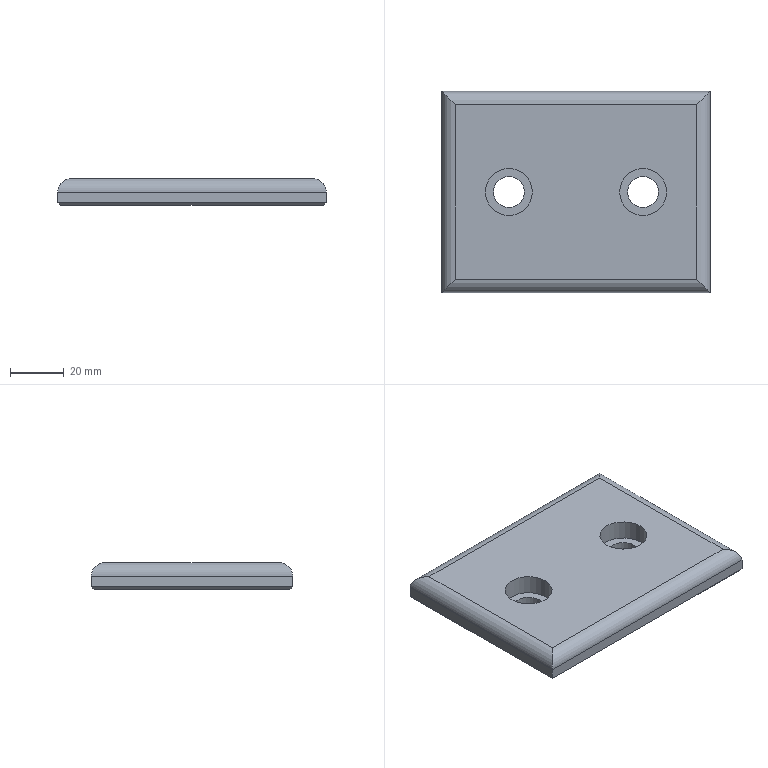Part | NX | features solid 2 | 1 solid | 20 faces | box 100 x 75 x 10 mm | volume 68924 mm3 | plane 12 | cylinder 8 | commonest cylinder face diameters 10 x4 11.5 x2 17.5 x2
STEP:
#1=CARTESIAN_POINT('',(660.,-700.,-129.));
#2=VERTEX_POINT('',#1);
#3=CARTESIAN_POINT('',(660.,-700.,-125.));
#4=VERTEX_POINT('',#3);
#5=CARTESIAN_POINT('',(660.,-700.,-130.));
#6=DIRECTION('',(0.,0.,1.));
#7=VECTOR('',#6,1000.);
#8=LINE('',#5,#7);
#9=EDGE_CURVE('',#2,#4,#8,.T.);
#10=ORIENTED_EDGE('',*,*,#9,.T.);
#11=CARTESIAN_POINT('',(660.,-625.,-125.));
#12=VERTEX_POINT('',#11);
#13=CARTESIAN_POINT('',(660.,-700.,-125.));
#14=DIRECTION('',(0.,-1.,0.));
#15=VECTOR('',#14,1000.);
#16=LINE('',#13,#15);
#17=EDGE_CURVE('',#12,#4,#16,.T.);
#18=ORIENTED_EDGE('',*,*,#17,.F.);
#19=CARTESIAN_POINT('',(660.,-625.,-129.));
#20=VERTEX_POINT('',#19);
#21=CARTESIAN_POINT('',(660.,-625.,-130.));
#22=DIRECTION('',(0.,0.,1.));
#23=VECTOR('',#22,1000.);
#24=LINE('',#21,#23);
#25=EDGE_CURVE('',#20,#12,#24,.T.);
#26=ORIENTED_EDGE('',*,*,#25,.F.);
#27=CARTESIAN_POINT('',(660.,-625.,-129.));
#28=DIRECTION('',(0.,1.,0.));
#29=VECTOR('',#28,1000.);
#30=LINE('',#27,#29);
#31=EDGE_CURVE('',#2,#20,#30,.T.);
#32=ORIENTED_EDGE('',*,*,#31,.F.);
#33=EDGE_LOOP('',(#10,#18,#26,#32));
#34=FACE_BOUND('',#33,.T.);
#35=CARTESIAN_POINT('',(660.,-625.,-130.));
#36=DIRECTION('',(1.,0.,0.));
#37=DIRECTION('',(0.,-1.,0.));
#38=AXIS2_PLACEMENT_3D('',#35,#36,#37);
#39=PLANE('',#38);
#40=ADVANCED_FACE('',(#34),#39,.F.);
#41=CARTESIAN_POINT('',(760.,-700.,-129.));
#42=VERTEX_POINT('',#41);
#43=CARTESIAN_POINT('',(760.,-700.,-125.));
#44=VERTEX_POINT('',#43);
#45=CARTESIAN_POINT('',(760.,-700.,-130.));
#46=DIRECTION('',(0.,0.,1.));
#47=VECTOR('',#46,1000.);
#48=LINE('',#45,#47);
#49=EDGE_CURVE('',#42,#44,#48,.T.);
#50=ORIENTED_EDGE('',*,*,#49,.T.);
#51=CARTESIAN_POINT('',(760.,-700.,-125.));
#52=DIRECTION('',(1.,0.,0.));
#53=VECTOR('',#52,1000.);
#54=LINE('',#51,#53);
#55=EDGE_CURVE('',#4,#44,#54,.T.);
#56=ORIENTED_EDGE('',*,*,#55,.F.);
#57=ORIENTED_EDGE('',*,*,#9,.F.);
#58=CARTESIAN_POINT('',(660.,-700.,-129.));
#59=DIRECTION('',(-1.,0.,0.));
#60=VECTOR('',#59,1000.);
#61=LINE('',#58,#60);
#62=EDGE_CURVE('',#42,#2,#61,.T.);
#63=ORIENTED_EDGE('',*,*,#62,.F.);
#64=EDGE_LOOP('',(#50,#56,#57,#63));
#65=FACE_BOUND('',#64,.T.);
#66=CARTESIAN_POINT('',(660.,-700.,-130.));
#67=DIRECTION('',(0.,1.,0.));
#68=DIRECTION('',(1.,0.,0.));
#69=AXIS2_PLACEMENT_3D('',#66,#67,#68);
#70=PLANE('',#69);
#71=ADVANCED_FACE('',(#65),#70,.F.);
#72=CARTESIAN_POINT('',(760.,-625.,-129.));
#73=VERTEX_POINT('',#72);
#74=CARTESIAN_POINT('',(760.,-625.,-125.));
#75=VERTEX_POINT('',#74);
#76=CARTESIAN_POINT('',(760.,-625.,-130.));
#77=DIRECTION('',(0.,0.,1.));
#78=VECTOR('',#77,1000.);
#79=LINE('',#76,#78);
#80=EDGE_CURVE('',#73,#75,#79,.T.);
#81=ORIENTED_EDGE('',*,*,#80,.T.);
#82=CARTESIAN_POINT('',(760.,-625.,-125.));
#83=DIRECTION('',(0.,1.,0.));
#84=VECTOR('',#83,1000.);
#85=LINE('',#82,#84);
#86=EDGE_CURVE('',#44,#75,#85,.T.);
#87=ORIENTED_EDGE('',*,*,#86,.F.);
#88=ORIENTED_EDGE('',*,*,#49,.F.);
#89=CARTESIAN_POINT('',(760.,-700.,-129.));
#90=DIRECTION('',(0.,-1.,0.));
#91=VECTOR('',#90,1000.);
#92=LINE('',#89,#91);
#93=EDGE_CURVE('',#73,#42,#92,.T.);
#94=ORIENTED_EDGE('',*,*,#93,.F.);
#95=EDGE_LOOP('',(#81,#87,#88,#94));
#96=FACE_BOUND('',#95,.T.);
#97=CARTESIAN_POINT('',(760.,-700.,-130.));
#98=DIRECTION('',(-1.,0.,0.));
#99=DIRECTION('',(0.,1.,0.));
#100=AXIS2_PLACEMENT_3D('',#97,#98,#99);
#101=PLANE('',#100);
#102=ADVANCED_FACE('',(#96),#101,.F.);
#103=ORIENTED_EDGE('',*,*,#25,.T.);
#104=CARTESIAN_POINT('',(660.,-625.,-125.));
#105=DIRECTION('',(-1.,0.,0.));
#106=VECTOR('',#105,1000.);
#107=LINE('',#104,#106);
#108=EDGE_CURVE('',#75,#12,#107,.T.);
#109=ORIENTED_EDGE('',*,*,#108,.F.);
#110=ORIENTED_EDGE('',*,*,#80,.F.);
#111=CARTESIAN_POINT('',(760.,-625.,-129.));
#112=DIRECTION('',(1.,0.,0.));
#113=VECTOR('',#112,1000.);
#114=LINE('',#111,#113);
#115=EDGE_CURVE('',#20,#73,#114,.T.);
#116=ORIENTED_EDGE('',*,*,#115,.F.);
#117=EDGE_LOOP('',(#103,#109,#110,#116));
#118=FACE_BOUND('',#117,.T.);
#119=CARTESIAN_POINT('',(760.,-625.,-130.));
#120=DIRECTION('',(0.,-1.,0.));
#121=DIRECTION('',(-1.,0.,0.));
#122=AXIS2_PLACEMENT_3D('',#119,#120,#121);
#123=PLANE('',#122);
#124=ADVANCED_FACE('',(#118),#123,.F.);
#125=CARTESIAN_POINT('',(661.,-626.,-130.));
#126=VERTEX_POINT('',#125);
#127=CARTESIAN_POINT('',(661.,-699.,-130.));
#128=VERTEX_POINT('',#127);
#129=CARTESIAN_POINT('',(661.,-625.,-130.));
#130=DIRECTION('',(0.,-1.,0.));
#131=VECTOR('',#130,1000.);
#132=LINE('',#129,#131);
#133=EDGE_CURVE('',#126,#128,#132,.T.);
#134=ORIENTED_EDGE('',*,*,#133,.F.);
#135=CARTESIAN_POINT('',(759.,-626.,-130.));
#136=VERTEX_POINT('',#135);
#137=CARTESIAN_POINT('',(660.,-626.,-130.));
#138=DIRECTION('',(-1.,0.,0.));
#139=VECTOR('',#138,1000.);
#140=LINE('',#137,#139);
#141=EDGE_CURVE('',#136,#126,#140,.T.);
#142=ORIENTED_EDGE('',*,*,#141,.F.);
#143=CARTESIAN_POINT('',(759.,-699.,-130.));
#144=VERTEX_POINT('',#143);
#145=CARTESIAN_POINT('',(759.,-625.,-130.));
#146=DIRECTION('',(0.,1.,0.));
#147=VECTOR('',#146,1000.);
#148=LINE('',#145,#147);
#149=EDGE_CURVE('',#144,#136,#148,.T.);
#150=ORIENTED_EDGE('',*,*,#149,.F.);
#151=CARTESIAN_POINT('',(660.,-699.,-130.));
#152=DIRECTION('',(1.,0.,0.));
#153=VECTOR('',#152,1000.);
#154=LINE('',#151,#153);
#155=EDGE_CURVE('',#128,#144,#154,.T.);
#156=ORIENTED_EDGE('',*,*,#155,.F.);
#157=EDGE_LOOP('',(#134,#142,#150,#156));
#158=FACE_BOUND('',#157,.T.);
#159=CARTESIAN_POINT('',(740.75,-662.5,-130.));
#160=VERTEX_POINT('',#159);
#161=CARTESIAN_POINT('',(735.,-662.5,-130.));
#162=DIRECTION('',(0.,0.,-1.));
#163=DIRECTION('',(1.,0.,0.));
#164=AXIS2_PLACEMENT_3D('',#161,#162,#163);
#165=CIRCLE('',#164,5.75);
#166=EDGE_CURVE('',#160,#160,#165,.T.);
#167=ORIENTED_EDGE('',*,*,#166,.F.);
#168=EDGE_LOOP('',(#167));
#169=FACE_BOUND('',#168,.T.);
#170=CARTESIAN_POINT('',(690.75,-662.5,-130.));
#171=VERTEX_POINT('',#170);
#172=CARTESIAN_POINT('',(685.,-662.5,-130.));
#173=DIRECTION('',(0.,0.,-1.));
#174=DIRECTION('',(1.,0.,0.));
#175=AXIS2_PLACEMENT_3D('',#172,#173,#174);
#176=CIRCLE('',#175,5.75);
#177=EDGE_CURVE('',#171,#171,#176,.T.);
#178=ORIENTED_EDGE('',*,*,#177,.F.);
#179=EDGE_LOOP('',(#178));
#180=FACE_BOUND('',#179,.T.);
#181=CARTESIAN_POINT('',(660.,-625.,-130.));
#182=DIRECTION('',(0.,0.,1.));
#183=DIRECTION('',(1.,0.,0.));
#184=AXIS2_PLACEMENT_3D('',#181,#182,#183);
#185=PLANE('',#184);
#186=ADVANCED_FACE('',(#158,#169,#180),#185,.F.);
#187=CARTESIAN_POINT('',(755.,-630.,-120.));
#188=VERTEX_POINT('',#187);
#189=CARTESIAN_POINT('',(755.,-695.,-120.));
#190=VERTEX_POINT('',#189);
#191=CARTESIAN_POINT('',(755.,-700.,-120.));
#192=DIRECTION('',(0.,1.,0.));
#193=VECTOR('',#192,1000.);
#194=LINE('',#191,#193);
#195=EDGE_CURVE('',#188,#190,#194,.F.);
#196=ORIENTED_EDGE('',*,*,#195,.F.);
#197=CARTESIAN_POINT('',(665.,-630.,-120.));
#198=VERTEX_POINT('',#197);
#199=CARTESIAN_POINT('',(760.,-630.,-120.));
#200=DIRECTION('',(-1.,0.,0.));
#201=VECTOR('',#200,1000.);
#202=LINE('',#199,#201);
#203=EDGE_CURVE('',#198,#188,#202,.F.);
#204=ORIENTED_EDGE('',*,*,#203,.F.);
#205=CARTESIAN_POINT('',(665.,-695.,-120.));
#206=VERTEX_POINT('',#205);
#207=CARTESIAN_POINT('',(665.,-625.,-120.));
#208=DIRECTION('',(0.,-1.,0.));
#209=VECTOR('',#208,1000.);
#210=LINE('',#207,#209);
#211=EDGE_CURVE('',#206,#198,#210,.F.);
#212=ORIENTED_EDGE('',*,*,#211,.F.);
#213=CARTESIAN_POINT('',(660.,-695.,-120.));
#214=DIRECTION('',(1.,0.,0.));
#215=VECTOR('',#214,1000.);
#216=LINE('',#213,#215);
#217=EDGE_CURVE('',#190,#206,#216,.F.);
#218=ORIENTED_EDGE('',*,*,#217,.F.);
#219=EDGE_LOOP('',(#196,#204,#212,#218));
#220=FACE_BOUND('',#219,.T.);
#221=CARTESIAN_POINT('',(726.25,-662.5,-120.));
#222=VERTEX_POINT('',#221);
#223=CARTESIAN_POINT('',(735.,-662.5,-120.));
#224=DIRECTION('',(0.,0.,1.));
#225=DIRECTION('',(-1.,0.,0.));
#226=AXIS2_PLACEMENT_3D('',#223,#224,#225);
#227=CIRCLE('',#226,8.75);
#228=EDGE_CURVE('',#222,#222,#227,.T.);
#229=ORIENTED_EDGE('',*,*,#228,.F.);
#230=EDGE_LOOP('',(#229));
#231=FACE_BOUND('',#230,.T.);
#232=CARTESIAN_POINT('',(676.25,-662.5,-120.));
#233=VERTEX_POINT('',#232);
#234=CARTESIAN_POINT('',(685.,-662.5,-120.));
#235=DIRECTION('',(0.,0.,1.));
#236=DIRECTION('',(-1.,0.,0.));
#237=AXIS2_PLACEMENT_3D('',#234,#235,#236);
#238=CIRCLE('',#237,8.75);
#239=EDGE_CURVE('',#233,#233,#238,.T.);
#240=ORIENTED_EDGE('',*,*,#239,.F.);
#241=EDGE_LOOP('',(#240));
#242=FACE_BOUND('',#241,.T.);
#243=CARTESIAN_POINT('',(660.,-625.,-120.));
#244=DIRECTION('',(0.,0.,1.));
#245=DIRECTION('',(1.,0.,0.));
#246=AXIS2_PLACEMENT_3D('',#243,#244,#245);
#247=PLANE('',#246);
#248=ADVANCED_FACE('',(#220,#231,#242),#247,.T.);
#249=CARTESIAN_POINT('',(679.25,-662.5,-127.3));
#250=VERTEX_POINT('',#249);
#251=CARTESIAN_POINT('',(685.,-662.5,-127.3));
#252=DIRECTION('',(0.,0.,1.));
#253=DIRECTION('',(-1.,0.,0.));
#254=AXIS2_PLACEMENT_3D('',#251,#252,#253);
#255=CIRCLE('',#254,5.75);
#256=EDGE_CURVE('',#250,#250,#255,.T.);
#257=ORIENTED_EDGE('',*,*,#256,.T.);
#258=EDGE_LOOP('',(#257));
#259=FACE_BOUND('',#258,.T.);
#260=ORIENTED_EDGE('',*,*,#177,.T.);
#261=EDGE_LOOP('',(#260));
#262=FACE_BOUND('',#261,.T.);
#263=CARTESIAN_POINT('',(685.,-662.5,-170.));
#264=DIRECTION('',(0.,0.,-1.));
#265=DIRECTION('',(-1.,0.,0.));
#266=AXIS2_PLACEMENT_3D('',#263,#264,#265);
#267=CYLINDRICAL_SURFACE('',#266,5.75);
#268=ADVANCED_FACE('',(#259,#262),#267,.F.);
#269=ORIENTED_EDGE('',*,*,#256,.F.);
#270=EDGE_LOOP('',(#269));
#271=FACE_BOUND('',#270,.T.);
#272=CARTESIAN_POINT('',(676.25,-662.5,-127.3));
#273=VERTEX_POINT('',#272);
#274=CARTESIAN_POINT('',(685.,-662.5,-127.3));
#275=DIRECTION('',(0.,0.,1.));
#276=DIRECTION('',(-1.,0.,0.));
#277=AXIS2_PLACEMENT_3D('',#274,#275,#276);
#278=CIRCLE('',#277,8.75);
#279=EDGE_CURVE('',#273,#273,#278,.T.);
#280=ORIENTED_EDGE('',*,*,#279,.T.);
#281=EDGE_LOOP('',(#280));
#282=FACE_BOUND('',#281,.T.);
#283=CARTESIAN_POINT('',(685.,-662.5,-127.3));
#284=DIRECTION('',(0.,0.,-1.));
#285=DIRECTION('',(-1.,0.,0.));
#286=AXIS2_PLACEMENT_3D('',#283,#284,#285);
#287=PLANE('',#286);
#288=ADVANCED_FACE('',(#271,#282),#287,.F.);
#289=ORIENTED_EDGE('',*,*,#279,.F.);
#290=EDGE_LOOP('',(#289));
#291=FACE_BOUND('',#290,.T.);
#292=ORIENTED_EDGE('',*,*,#239,.T.);
#293=EDGE_LOOP('',(#292));
#294=FACE_BOUND('',#293,.T.);
#295=CARTESIAN_POINT('',(685.,-662.5,-120.));
#296=DIRECTION('',(0.,0.,-1.));
#297=DIRECTION('',(-1.,0.,0.));
#298=AXIS2_PLACEMENT_3D('',#295,#296,#297);
#299=CYLINDRICAL_SURFACE('',#298,8.75);
#300=ADVANCED_FACE('',(#291,#294),#299,.F.);
#301=CARTESIAN_POINT('',(729.25,-662.5,-127.3));
#302=VERTEX_POINT('',#301);
#303=CARTESIAN_POINT('',(735.,-662.5,-127.3));
#304=DIRECTION('',(0.,0.,1.));
#305=DIRECTION('',(-1.,0.,0.));
#306=AXIS2_PLACEMENT_3D('',#303,#304,#305);
#307=CIRCLE('',#306,5.75);
#308=EDGE_CURVE('',#302,#302,#307,.T.);
#309=ORIENTED_EDGE('',*,*,#308,.T.);
#310=EDGE_LOOP('',(#309));
#311=FACE_BOUND('',#310,.T.);
#312=ORIENTED_EDGE('',*,*,#166,.T.);
#313=EDGE_LOOP('',(#312));
#314=FACE_BOUND('',#313,.T.);
#315=CARTESIAN_POINT('',(735.,-662.5,-170.));
#316=DIRECTION('',(0.,0.,-1.));
#317=DIRECTION('',(-1.,0.,0.));
#318=AXIS2_PLACEMENT_3D('',#315,#316,#317);
#319=CYLINDRICAL_SURFACE('',#318,5.75);
#320=ADVANCED_FACE('',(#311,#314),#319,.F.);
#321=ORIENTED_EDGE('',*,*,#308,.F.);
#322=EDGE_LOOP('',(#321));
#323=FACE_BOUND('',#322,.T.);
#324=CARTESIAN_POINT('',(726.25,-662.5,-127.3));
#325=VERTEX_POINT('',#324);
#326=CARTESIAN_POINT('',(735.,-662.5,-127.3));
#327=DIRECTION('',(0.,0.,1.));
#328=DIRECTION('',(-1.,0.,0.));
#329=AXIS2_PLACEMENT_3D('',#326,#327,#328);
#330=CIRCLE('',#329,8.75);
#331=EDGE_CURVE('',#325,#325,#330,.T.);
#332=ORIENTED_EDGE('',*,*,#331,.T.);
#333=EDGE_LOOP('',(#332));
#334=FACE_BOUND('',#333,.T.);
#335=CARTESIAN_POINT('',(735.,-662.5,-127.3));
#336=DIRECTION('',(0.,0.,-1.));
#337=DIRECTION('',(-1.,0.,0.));
#338=AXIS2_PLACEMENT_3D('',#335,#336,#337);
#339=PLANE('',#338);
#340=ADVANCED_FACE('',(#323,#334),#339,.F.);
#341=ORIENTED_EDGE('',*,*,#331,.F.);
#342=EDGE_LOOP('',(#341));
#343=FACE_BOUND('',#342,.T.);
#344=ORIENTED_EDGE('',*,*,#228,.T.);
#345=EDGE_LOOP('',(#344));
#346=FACE_BOUND('',#345,.T.);
#347=CARTESIAN_POINT('',(735.,-662.5,-120.));
#348=DIRECTION('',(0.,0.,-1.));
#349=DIRECTION('',(-1.,0.,0.));
#350=AXIS2_PLACEMENT_3D('',#347,#348,#349);
#351=CYLINDRICAL_SURFACE('',#350,8.75);
#352=ADVANCED_FACE('',(#343,#346),#351,.F.);
#353=CARTESIAN_POINT('',(755.,-630.,-125.));
#354=DIRECTION('',(-0.7071,0.7071,0.));
#355=DIRECTION('',(0.7071,0.7071,0.));
#356=AXIS2_PLACEMENT_3D('',#353,#354,#355);
#357=ELLIPSE('',#356,7.071,5.);
#358=EDGE_CURVE('',#188,#75,#357,.T.);
#359=ORIENTED_EDGE('',*,*,#358,.T.);
#360=ORIENTED_EDGE('',*,*,#108,.T.);
#361=CARTESIAN_POINT('',(665.,-630.,-125.));
#362=DIRECTION('',(-0.7071,-0.7071,0.));
#363=DIRECTION('',(-0.7071,0.7071,0.));
#364=AXIS2_PLACEMENT_3D('',#361,#362,#363);
#365=ELLIPSE('',#364,7.071,5.);
#366=EDGE_CURVE('',#12,#198,#365,.F.);
#367=ORIENTED_EDGE('',*,*,#366,.T.);
#368=ORIENTED_EDGE('',*,*,#203,.T.);
#369=EDGE_LOOP('',(#359,#360,#367,#368));
#370=FACE_BOUND('',#369,.T.);
#371=CARTESIAN_POINT('',(760.,-630.,-125.));
#372=DIRECTION('',(1.,0.,0.));
#373=DIRECTION('',(0.,-1.,0.));
#374=AXIS2_PLACEMENT_3D('',#371,#372,#373);
#375=CYLINDRICAL_SURFACE('',#374,5.);
#376=ADVANCED_FACE('',(#370),#375,.T.);
#377=ORIENTED_EDGE('',*,*,#366,.F.);
#378=ORIENTED_EDGE('',*,*,#17,.T.);
#379=CARTESIAN_POINT('',(665.,-695.,-125.));
#380=DIRECTION('',(0.7071,-0.7071,0.));
#381=DIRECTION('',(0.7071,0.7071,0.));
#382=AXIS2_PLACEMENT_3D('',#379,#380,#381);
#383=ELLIPSE('',#382,7.071,5.);
#384=EDGE_CURVE('',#4,#206,#383,.F.);
#385=ORIENTED_EDGE('',*,*,#384,.T.);
#386=ORIENTED_EDGE('',*,*,#211,.T.);
#387=EDGE_LOOP('',(#377,#378,#385,#386));
#388=FACE_BOUND('',#387,.T.);
#389=CARTESIAN_POINT('',(665.,-625.,-125.));
#390=DIRECTION('',(0.,1.,0.));
#391=DIRECTION('',(1.,0.,0.));
#392=AXIS2_PLACEMENT_3D('',#389,#390,#391);
#393=CYLINDRICAL_SURFACE('',#392,5.);
#394=ADVANCED_FACE('',(#388),#393,.T.);
#395=ORIENTED_EDGE('',*,*,#358,.F.);
#396=ORIENTED_EDGE('',*,*,#195,.T.);
#397=CARTESIAN_POINT('',(755.,-695.,-125.));
#398=DIRECTION('',(0.7071,0.7071,0.));
#399=DIRECTION('',(0.7071,-0.7071,0.));
#400=AXIS2_PLACEMENT_3D('',#397,#398,#399);
#401=ELLIPSE('',#400,7.071,5.);
#402=EDGE_CURVE('',#190,#44,#401,.T.);
#403=ORIENTED_EDGE('',*,*,#402,.T.);
#404=ORIENTED_EDGE('',*,*,#86,.T.);
#405=EDGE_LOOP('',(#395,#396,#403,#404));
#406=FACE_BOUND('',#405,.T.);
#407=CARTESIAN_POINT('',(755.,-700.,-125.));
#408=DIRECTION('',(0.,-1.,0.));
#409=DIRECTION('',(-1.,0.,0.));
#410=AXIS2_PLACEMENT_3D('',#407,#408,#409);
#411=CYLINDRICAL_SURFACE('',#410,5.);
#412=ADVANCED_FACE('',(#406),#411,.T.);
#413=ORIENTED_EDGE('',*,*,#384,.F.);
#414=ORIENTED_EDGE('',*,*,#55,.T.);
#415=ORIENTED_EDGE('',*,*,#402,.F.);
#416=ORIENTED_EDGE('',*,*,#217,.T.);
#417=EDGE_LOOP('',(#413,#414,#415,#416));
#418=FACE_BOUND('',#417,.T.);
#419=CARTESIAN_POINT('',(660.,-695.,-125.));
#420=DIRECTION('',(-1.,0.,0.));
#421=DIRECTION('',(0.,1.,0.));
#422=AXIS2_PLACEMENT_3D('',#419,#420,#421);
#423=CYLINDRICAL_SURFACE('',#422,5.);
#424=ADVANCED_FACE('',(#418),#423,.T.);
#425=CARTESIAN_POINT('',(726.,-659.,-163.));
#426=DIRECTION('',(0.5774,0.5774,0.5774));
#427=VECTOR('',#426,1000.);
#428=LINE('',#425,#427);
#429=EDGE_CURVE('',#73,#136,#428,.F.);
#430=ORIENTED_EDGE('',*,*,#429,.T.);
#431=ORIENTED_EDGE('',*,*,#141,.T.);
#432=CARTESIAN_POINT('',(660.667,-625.667,-129.667));
#433=DIRECTION('',(-0.5774,0.5774,0.5774));
#434=VECTOR('',#433,1000.);
#435=LINE('',#432,#434);
#436=EDGE_CURVE('',#126,#20,#435,.T.);
#437=ORIENTED_EDGE('',*,*,#436,.T.);
#438=ORIENTED_EDGE('',*,*,#115,.T.);
#439=EDGE_LOOP('',(#430,#431,#437,#438));
#440=FACE_BOUND('',#439,.T.);
#441=CARTESIAN_POINT('',(660.,-626.,-130.));
#442=DIRECTION('',(0.,-0.7071,0.7071));
#443=DIRECTION('',(0.,0.7071,0.7071));
#444=AXIS2_PLACEMENT_3D('',#441,#442,#443);
#445=PLANE('',#444);
#446=ADVANCED_FACE('',(#440),#445,.F.);
#447=ORIENTED_EDGE('',*,*,#436,.F.);
#448=ORIENTED_EDGE('',*,*,#133,.T.);
#449=CARTESIAN_POINT('',(685.667,-674.333,-154.667));
#450=DIRECTION('',(0.5774,0.5774,-0.5774));
#451=VECTOR('',#450,1000.);
#452=LINE('',#449,#451);
#453=EDGE_CURVE('',#128,#2,#452,.F.);
#454=ORIENTED_EDGE('',*,*,#453,.T.);
#455=ORIENTED_EDGE('',*,*,#31,.T.);
#456=EDGE_LOOP('',(#447,#448,#454,#455));
#457=FACE_BOUND('',#456,.T.);
#458=CARTESIAN_POINT('',(661.,-625.,-130.));
#459=DIRECTION('',(0.7071,0.,0.7071));
#460=DIRECTION('',(0.7071,0.,-0.7071));
#461=AXIS2_PLACEMENT_3D('',#458,#459,#460);
#462=PLANE('',#461);
#463=ADVANCED_FACE('',(#457),#462,.F.);
#464=ORIENTED_EDGE('',*,*,#429,.F.);
#465=ORIENTED_EDGE('',*,*,#93,.T.);
#466=CARTESIAN_POINT('',(734.333,-674.333,-154.667));
#467=DIRECTION('',(0.5774,-0.5774,0.5774));
#468=VECTOR('',#467,1000.);
#469=LINE('',#466,#468);
#470=EDGE_CURVE('',#42,#144,#469,.F.);
#471=ORIENTED_EDGE('',*,*,#470,.T.);
#472=ORIENTED_EDGE('',*,*,#149,.T.);
#473=EDGE_LOOP('',(#464,#465,#471,#472));
#474=FACE_BOUND('',#473,.T.);
#475=CARTESIAN_POINT('',(759.,-625.,-130.));
#476=DIRECTION('',(-0.7071,0.,0.7071));
#477=DIRECTION('',(0.7071,0.,0.7071));
#478=AXIS2_PLACEMENT_3D('',#475,#476,#477);
#479=PLANE('',#478);
#480=ADVANCED_FACE('',(#474),#479,.F.);
#481=ORIENTED_EDGE('',*,*,#453,.F.);
#482=ORIENTED_EDGE('',*,*,#155,.T.);
#483=ORIENTED_EDGE('',*,*,#470,.F.);
#484=ORIENTED_EDGE('',*,*,#62,.T.);
#485=EDGE_LOOP('',(#481,#482,#483,#484));
#486=FACE_BOUND('',#485,.T.);
#487=CARTESIAN_POINT('',(660.,-699.,-130.));
#488=DIRECTION('',(0.,0.7071,0.7071));
#489=DIRECTION('',(0.,0.7071,-0.7071));
#490=AXIS2_PLACEMENT_3D('',#487,#488,#489);
#491=PLANE('',#490);
#492=ADVANCED_FACE('',(#486),#491,.F.);
#493=CLOSED_SHELL('',(#40,#71,#102,#124,#186,#248,#268,#288,#300,#320,#340,#352,#376,#394,#412,#424,#446,#463,#480,#492));
#494=MANIFOLD_SOLID_BREP('',#493);
#495=(LENGTH_UNIT()NAMED_UNIT(*)SI_UNIT(.MILLI.,.METRE.));
#496=UNCERTAINTY_MEASURE_WITH_UNIT(LENGTH_MEASURE(0.00001),#495,'','');
#497=(NAMED_UNIT(*)PLANE_ANGLE_UNIT()SI_UNIT($,.RADIAN.));
#498=(NAMED_UNIT(*)SI_UNIT($,.STERADIAN.)SOLID_ANGLE_UNIT());
#499=(GEOMETRIC_REPRESENTATION_CONTEXT(3)GLOBAL_UNCERTAINTY_ASSIGNED_CONTEXT((#496))GLOBAL_UNIT_ASSIGNED_CONTEXT((#495,#497,#498))REPRESENTATION_CONTEXT('',''));
#500=ADVANCED_BREP_SHAPE_REPRESENTATION('',(#494),#499);